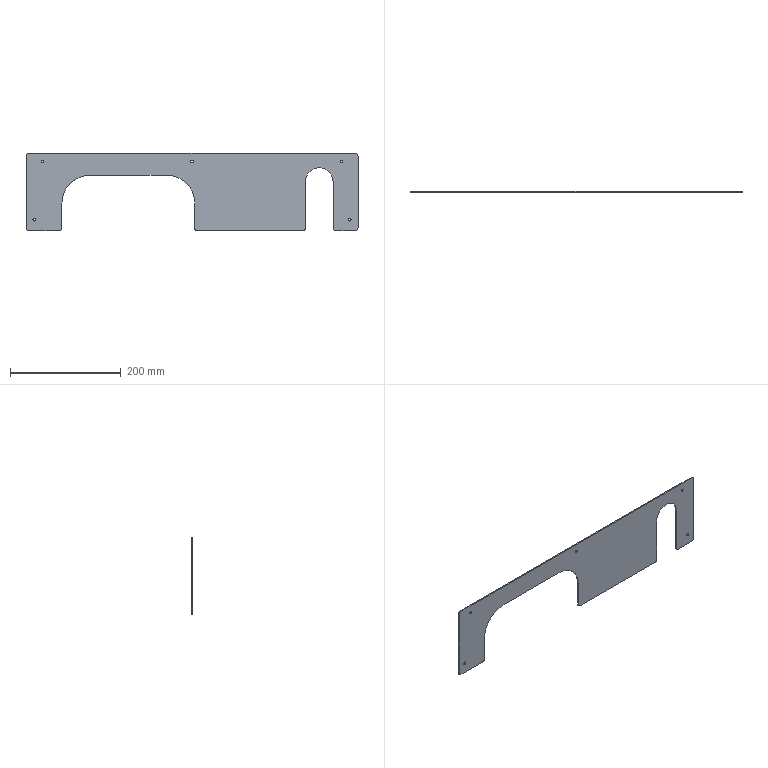Part | STEP file | CHAIN.COVER.2.stp | 1 solid | 44 faces | box 600 x 2 x 140 mm | volume 111000 mm3 | cylinder 27 | spline 13 | plane 4 | commonest cylinder face diameters 10 x16 5 x6 100 x4 50 x1